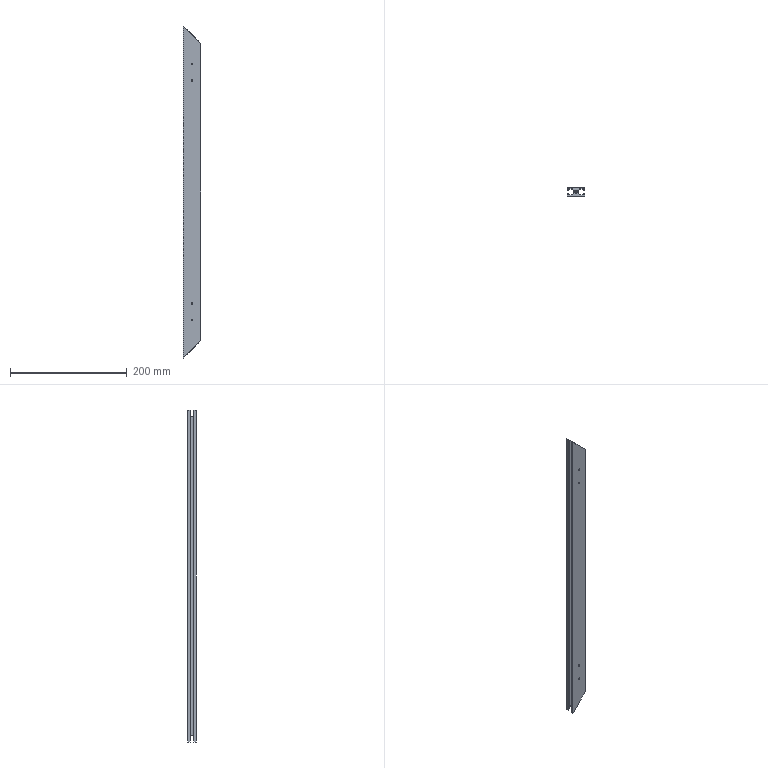Part | SolidWorks | features Extrusion 1, HoleWzd 1, ICE 1 | 1 solid | 49 faces | box 30 x 15 x 568 mm | volume 128082 mm3 | cylinder 21 | plane 20 | cone 8 | commonest cylinder face diameters 3.3 x16 5 x2 16.345 x2 16.33 x1